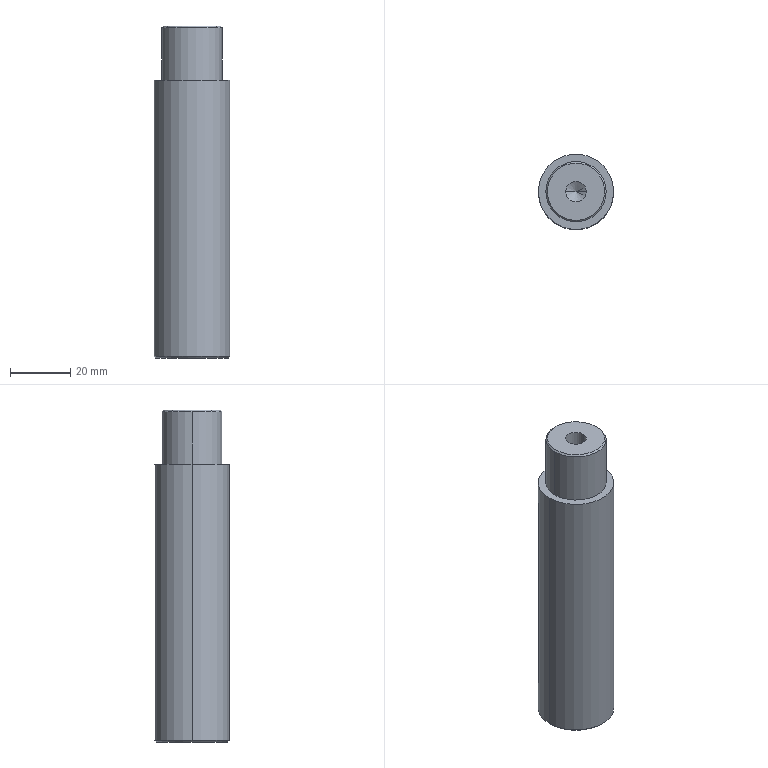Part | STEP file | 11-FG-Z00411 | 1 solid | 19 faces | box 25 x 25 x 110 mm | volume 49310 mm3 | cone 8 | cylinder 8 | plane 3 | commonest cylinder face diameters 6.8 x4 20 x2 25 x2
STEP:
#1=CARTESIAN_POINT('',(-12.,0.,0.));
#2=VERTEX_POINT('',#1);
#3=CARTESIAN_POINT('',(12.,0.,0.));
#4=VERTEX_POINT('',#3);
#5=CARTESIAN_POINT('',(0.,0.,0.));
#6=DIRECTION('',(0.,0.,-1.));
#7=DIRECTION('',(1.,0.,0.));
#8=AXIS2_PLACEMENT_3D('',#5,#6,#7);
#9=CIRCLE('',#8,12.);
#10=EDGE_CURVE('',#2,#4,#9,.T.);
#11=ORIENTED_EDGE('',*,*,#10,.F.);
#12=CARTESIAN_POINT('',(-12.5,0.,0.5));
#13=VERTEX_POINT('',#12);
#14=CARTESIAN_POINT('',(-12.5,0.,0.5));
#15=DIRECTION('',(-0.7071,0.,0.7071));
#16=VECTOR('',#15,1000.);
#17=LINE('',#14,#16);
#18=EDGE_CURVE('',#2,#13,#17,.T.);
#19=ORIENTED_EDGE('',*,*,#18,.T.);
#20=CARTESIAN_POINT('',(12.5,0.,0.5));
#21=VERTEX_POINT('',#20);
#22=CARTESIAN_POINT('',(0.,0.,0.5));
#23=DIRECTION('',(0.,0.,1.));
#24=DIRECTION('',(1.,0.,0.));
#25=AXIS2_PLACEMENT_3D('',#22,#23,#24);
#26=CIRCLE('',#25,12.5);
#27=EDGE_CURVE('',#21,#13,#26,.T.);
#28=ORIENTED_EDGE('',*,*,#27,.F.);
#29=CARTESIAN_POINT('',(12.5,0.,0.5));
#30=DIRECTION('',(0.7071,0.,0.7071));
#31=VECTOR('',#30,1000.);
#32=LINE('',#29,#31);
#33=EDGE_CURVE('',#4,#21,#32,.T.);
#34=ORIENTED_EDGE('',*,*,#33,.F.);
#35=EDGE_LOOP('',(#11,#19,#28,#34));
#36=FACE_OUTER_BOUND('',#35,.T.);
#37=CARTESIAN_POINT('',(0.,0.,0.5));
#38=DIRECTION('',(0.,0.,1.));
#39=DIRECTION('',(1.,0.,0.));
#40=AXIS2_PLACEMENT_3D('',#37,#38,#39);
#41=CONICAL_SURFACE('',#40,12.5,0.7854);
#42=ADVANCED_FACE('',(#36),#41,.T.);
#43=CARTESIAN_POINT('',(9.5,0.,110.));
#44=VERTEX_POINT('',#43);
#45=CARTESIAN_POINT('',(-9.5,0.,110.));
#46=VERTEX_POINT('',#45);
#47=CARTESIAN_POINT('',(0.,0.,110.));
#48=DIRECTION('',(0.,0.,1.));
#49=DIRECTION('',(1.,0.,0.));
#50=AXIS2_PLACEMENT_3D('',#47,#48,#49);
#51=CIRCLE('',#50,9.5);
#52=EDGE_CURVE('',#44,#46,#51,.T.);
#53=ORIENTED_EDGE('',*,*,#52,.F.);
#54=CARTESIAN_POINT('',(10.,0.,109.5));
#55=VERTEX_POINT('',#54);
#56=CARTESIAN_POINT('',(9.5,0.,110.));
#57=DIRECTION('',(0.7071,0.,-0.7071));
#58=VECTOR('',#57,1000.);
#59=LINE('',#56,#58);
#60=EDGE_CURVE('',#44,#55,#59,.T.);
#61=ORIENTED_EDGE('',*,*,#60,.T.);
#62=CARTESIAN_POINT('',(-10.,0.,109.5));
#63=VERTEX_POINT('',#62);
#64=CARTESIAN_POINT('',(0.,0.,109.5));
#65=DIRECTION('',(0.,0.,-1.));
#66=DIRECTION('',(1.,0.,0.));
#67=AXIS2_PLACEMENT_3D('',#64,#65,#66);
#68=CIRCLE('',#67,10.);
#69=EDGE_CURVE('',#63,#55,#68,.T.);
#70=ORIENTED_EDGE('',*,*,#69,.F.);
#71=CARTESIAN_POINT('',(-9.5,0.,110.));
#72=DIRECTION('',(-0.7071,0.,-0.7071));
#73=VECTOR('',#72,1000.);
#74=LINE('',#71,#73);
#75=EDGE_CURVE('',#46,#63,#74,.T.);
#76=ORIENTED_EDGE('',*,*,#75,.F.);
#77=EDGE_LOOP('',(#53,#61,#70,#76));
#78=FACE_OUTER_BOUND('',#77,.T.);
#79=CARTESIAN_POINT('',(0.,0.,110.));
#80=DIRECTION('',(0.,0.,-1.));
#81=DIRECTION('',(-1.,0.,0.));
#82=AXIS2_PLACEMENT_3D('',#79,#80,#81);
#83=CONICAL_SURFACE('',#82,9.5,0.7854);
#84=ADVANCED_FACE('',(#78),#83,.T.);
#85=CARTESIAN_POINT('',(-3.4,0.,90.2));
#86=VERTEX_POINT('',#85);
#87=CARTESIAN_POINT('',(3.4,0.,90.2));
#88=VERTEX_POINT('',#87);
#89=CARTESIAN_POINT('',(0.,0.,90.2));
#90=DIRECTION('',(0.,0.,1.));
#91=DIRECTION('',(1.,0.,0.));
#92=AXIS2_PLACEMENT_3D('',#89,#90,#91);
#93=CIRCLE('',#92,3.4);
#94=EDGE_CURVE('',#86,#88,#93,.T.);
#95=ORIENTED_EDGE('',*,*,#94,.F.);
#96=CARTESIAN_POINT('',(-3.4,0.,110.));
#97=VERTEX_POINT('',#96);
#98=CARTESIAN_POINT('',(-3.4,0.,110.));
#99=DIRECTION('',(0.,0.,1.));
#100=VECTOR('',#99,1000.);
#101=LINE('',#98,#100);
#102=EDGE_CURVE('',#86,#97,#101,.T.);
#103=ORIENTED_EDGE('',*,*,#102,.T.);
#104=CARTESIAN_POINT('',(3.4,0.,110.));
#105=VERTEX_POINT('',#104);
#106=CARTESIAN_POINT('',(0.,0.,110.));
#107=DIRECTION('',(0.,0.,1.));
#108=DIRECTION('',(1.,0.,0.));
#109=AXIS2_PLACEMENT_3D('',#106,#107,#108);
#110=CIRCLE('',#109,3.4);
#111=EDGE_CURVE('',#97,#105,#110,.T.);
#112=ORIENTED_EDGE('',*,*,#111,.T.);
#113=CARTESIAN_POINT('',(3.4,0.,110.));
#114=DIRECTION('',(0.,0.,1.));
#115=VECTOR('',#114,1000.);
#116=LINE('',#113,#115);
#117=EDGE_CURVE('',#88,#105,#116,.T.);
#118=ORIENTED_EDGE('',*,*,#117,.F.);
#119=EDGE_LOOP('',(#95,#103,#112,#118));
#120=FACE_OUTER_BOUND('',#119,.T.);
#121=CARTESIAN_POINT('',(0.,0.,110.));
#122=DIRECTION('',(0.,0.,1.));
#123=DIRECTION('',(1.,0.,0.));
#124=AXIS2_PLACEMENT_3D('',#121,#122,#123);
#125=CYLINDRICAL_SURFACE('',#124,3.4);
#126=ADVANCED_FACE('',(#120),#125,.F.);
#127=CARTESIAN_POINT('',(0.,0.,88.157));
#128=VERTEX_POINT('',#127);
#129=CARTESIAN_POINT('',(3.4,0.,90.2));
#130=DIRECTION('',(0.8572,0.,0.515));
#131=VECTOR('',#130,1000.);
#132=LINE('',#129,#131);
#133=EDGE_CURVE('',#128,#88,#132,.T.);
#134=ORIENTED_EDGE('',*,*,#133,.F.);
#135=CARTESIAN_POINT('',(-3.4,0.,90.2));
#136=DIRECTION('',(-0.8572,0.,0.515));
#137=VECTOR('',#136,1000.);
#138=LINE('',#135,#137);
#139=EDGE_CURVE('',#128,#86,#138,.T.);
#140=ORIENTED_EDGE('',*,*,#139,.T.);
#141=ORIENTED_EDGE('',*,*,#94,.T.);
#142=EDGE_LOOP('',(#134,#140,#141));
#143=FACE_OUTER_BOUND('',#142,.T.);
#144=CARTESIAN_POINT('',(0.,0.,90.2));
#145=DIRECTION('',(0.,0.,1.));
#146=DIRECTION('',(1.,0.,0.));
#147=AXIS2_PLACEMENT_3D('',#144,#145,#146);
#148=CONICAL_SURFACE('',#147,3.4,1.03);
#149=ADVANCED_FACE('',(#143),#148,.F.);
#150=CARTESIAN_POINT('',(10.,0.,92.));
#151=VERTEX_POINT('',#150);
#152=CARTESIAN_POINT('',(-10.,0.,92.));
#153=VERTEX_POINT('',#152);
#154=CARTESIAN_POINT('',(0.,0.,92.));
#155=DIRECTION('',(0.,0.,1.));
#156=DIRECTION('',(1.,0.,0.));
#157=AXIS2_PLACEMENT_3D('',#154,#155,#156);
#158=CIRCLE('',#157,10.);
#159=EDGE_CURVE('',#151,#153,#158,.T.);
#160=ORIENTED_EDGE('',*,*,#159,.T.);
#161=CARTESIAN_POINT('',(-10.,0.,92.));
#162=DIRECTION('',(0.,0.,1.));
#163=VECTOR('',#162,1000.);
#164=LINE('',#161,#163);
#165=EDGE_CURVE('',#153,#63,#164,.T.);
#166=ORIENTED_EDGE('',*,*,#165,.T.);
#167=ORIENTED_EDGE('',*,*,#69,.T.);
#168=CARTESIAN_POINT('',(10.,0.,92.));
#169=DIRECTION('',(0.,0.,1.));
#170=VECTOR('',#169,1000.);
#171=LINE('',#168,#170);
#172=EDGE_CURVE('',#151,#55,#171,.T.);
#173=ORIENTED_EDGE('',*,*,#172,.F.);
#174=EDGE_LOOP('',(#160,#166,#167,#173));
#175=FACE_OUTER_BOUND('',#174,.T.);
#176=CARTESIAN_POINT('',(0.,0.,92.));
#177=DIRECTION('',(0.,0.,1.));
#178=DIRECTION('',(1.,0.,0.));
#179=AXIS2_PLACEMENT_3D('',#176,#177,#178);
#180=CYLINDRICAL_SURFACE('',#179,10.);
#181=ADVANCED_FACE('',(#175),#180,.T.);
#182=CARTESIAN_POINT('',(3.4,0.,19.8));
#183=VERTEX_POINT('',#182);
#184=CARTESIAN_POINT('',(-3.4,0.,19.8));
#185=VERTEX_POINT('',#184);
#186=CARTESIAN_POINT('',(0.,0.,19.8));
#187=DIRECTION('',(0.,0.,-1.));
#188=DIRECTION('',(-1.,0.,0.));
#189=AXIS2_PLACEMENT_3D('',#186,#187,#188);
#190=CIRCLE('',#189,3.4);
#191=EDGE_CURVE('',#183,#185,#190,.T.);
#192=ORIENTED_EDGE('',*,*,#191,.F.);
#193=CARTESIAN_POINT('',(3.4,0.,0.));
#194=VERTEX_POINT('',#193);
#195=CARTESIAN_POINT('',(3.4,0.,0.));
#196=DIRECTION('',(0.,0.,-1.));
#197=VECTOR('',#196,1000.);
#198=LINE('',#195,#197);
#199=EDGE_CURVE('',#183,#194,#198,.T.);
#200=ORIENTED_EDGE('',*,*,#199,.T.);
#201=CARTESIAN_POINT('',(-3.4,0.,0.));
#202=VERTEX_POINT('',#201);
#203=CARTESIAN_POINT('',(0.,0.,0.));
#204=DIRECTION('',(0.,0.,-1.));
#205=DIRECTION('',(-1.,0.,0.));
#206=AXIS2_PLACEMENT_3D('',#203,#204,#205);
#207=CIRCLE('',#206,3.4);
#208=EDGE_CURVE('',#194,#202,#207,.T.);
#209=ORIENTED_EDGE('',*,*,#208,.T.);
#210=CARTESIAN_POINT('',(-3.4,0.,0.));
#211=DIRECTION('',(0.,0.,-1.));
#212=VECTOR('',#211,1000.);
#213=LINE('',#210,#212);
#214=EDGE_CURVE('',#185,#202,#213,.T.);
#215=ORIENTED_EDGE('',*,*,#214,.F.);
#216=EDGE_LOOP('',(#192,#200,#209,#215));
#217=FACE_OUTER_BOUND('',#216,.T.);
#218=CARTESIAN_POINT('',(0.,0.,0.));
#219=DIRECTION('',(0.,0.,-1.));
#220=DIRECTION('',(-1.,0.,0.));
#221=AXIS2_PLACEMENT_3D('',#218,#219,#220);
#222=CYLINDRICAL_SURFACE('',#221,3.4);
#223=ADVANCED_FACE('',(#217),#222,.F.);
#224=CARTESIAN_POINT('',(0.,0.,21.843));
#225=VERTEX_POINT('',#224);
#226=CARTESIAN_POINT('',(-3.4,0.,19.8));
#227=DIRECTION('',(-0.8572,0.,-0.515));
#228=VECTOR('',#227,1000.);
#229=LINE('',#226,#228);
#230=EDGE_CURVE('',#225,#185,#229,.T.);
#231=ORIENTED_EDGE('',*,*,#230,.F.);
#232=CARTESIAN_POINT('',(3.4,0.,19.8));
#233=DIRECTION('',(0.8572,0.,-0.515));
#234=VECTOR('',#233,1000.);
#235=LINE('',#232,#234);
#236=EDGE_CURVE('',#225,#183,#235,.T.);
#237=ORIENTED_EDGE('',*,*,#236,.T.);
#238=ORIENTED_EDGE('',*,*,#191,.T.);
#239=EDGE_LOOP('',(#231,#237,#238));
#240=FACE_OUTER_BOUND('',#239,.T.);
#241=CARTESIAN_POINT('',(0.,0.,19.8));
#242=DIRECTION('',(0.,0.,-1.));
#243=DIRECTION('',(-1.,0.,0.));
#244=AXIS2_PLACEMENT_3D('',#241,#242,#243);
#245=CONICAL_SURFACE('',#244,3.4,1.03);
#246=ADVANCED_FACE('',(#240),#245,.F.);
#247=CARTESIAN_POINT('',(12.5,0.,92.));
#248=VERTEX_POINT('',#247);
#249=CARTESIAN_POINT('',(-12.5,0.,92.));
#250=VERTEX_POINT('',#249);
#251=CARTESIAN_POINT('',(0.,0.,92.));
#252=DIRECTION('',(0.,0.,1.));
#253=DIRECTION('',(1.,0.,0.));
#254=AXIS2_PLACEMENT_3D('',#251,#252,#253);
#255=CIRCLE('',#254,12.5);
#256=EDGE_CURVE('',#248,#250,#255,.T.);
#257=ORIENTED_EDGE('',*,*,#256,.F.);
#258=CARTESIAN_POINT('',(12.5,0.,110.));
#259=DIRECTION('',(0.,0.,-1.));
#260=VECTOR('',#259,1000.);
#261=LINE('',#258,#260);
#262=EDGE_CURVE('',#248,#21,#261,.T.);
#263=ORIENTED_EDGE('',*,*,#262,.T.);
#264=ORIENTED_EDGE('',*,*,#27,.T.);
#265=CARTESIAN_POINT('',(-12.5,0.,110.));
#266=DIRECTION('',(0.,0.,-1.));
#267=VECTOR('',#266,1000.);
#268=LINE('',#265,#267);
#269=EDGE_CURVE('',#250,#13,#268,.T.);
#270=ORIENTED_EDGE('',*,*,#269,.F.);
#271=EDGE_LOOP('',(#257,#263,#264,#270));
#272=FACE_OUTER_BOUND('',#271,.T.);
#273=CARTESIAN_POINT('',(0.,0.,110.));
#274=DIRECTION('',(0.,0.,-1.));
#275=DIRECTION('',(-1.,0.,0.));
#276=AXIS2_PLACEMENT_3D('',#273,#274,#275);
#277=CYLINDRICAL_SURFACE('',#276,12.5);
#278=ADVANCED_FACE('',(#272),#277,.T.);
#279=ORIENTED_EDGE('',*,*,#262,.F.);
#280=CARTESIAN_POINT('',(0.,0.,92.));
#281=DIRECTION('',(0.,0.,1.));
#282=DIRECTION('',(1.,0.,0.));
#283=AXIS2_PLACEMENT_3D('',#280,#281,#282);
#284=CIRCLE('',#283,12.5);
#285=EDGE_CURVE('',#250,#248,#284,.T.);
#286=ORIENTED_EDGE('',*,*,#285,.F.);
#287=ORIENTED_EDGE('',*,*,#269,.T.);
#288=CARTESIAN_POINT('',(0.,0.,0.5));
#289=DIRECTION('',(0.,0.,1.));
#290=DIRECTION('',(1.,0.,0.));
#291=AXIS2_PLACEMENT_3D('',#288,#289,#290);
#292=CIRCLE('',#291,12.5);
#293=EDGE_CURVE('',#13,#21,#292,.T.);
#294=ORIENTED_EDGE('',*,*,#293,.T.);
#295=EDGE_LOOP('',(#279,#286,#287,#294));
#296=FACE_OUTER_BOUND('',#295,.T.);
#297=CARTESIAN_POINT('',(0.,0.,110.));
#298=DIRECTION('',(0.,0.,-1.));
#299=DIRECTION('',(-1.,0.,0.));
#300=AXIS2_PLACEMENT_3D('',#297,#298,#299);
#301=CYLINDRICAL_SURFACE('',#300,12.5);
#302=ADVANCED_FACE('',(#296),#301,.T.);
#303=CARTESIAN_POINT('',(0.,0.,0.));
#304=DIRECTION('',(0.,0.,-1.));
#305=DIRECTION('',(1.,0.,0.));
#306=AXIS2_PLACEMENT_3D('',#303,#304,#305);
#307=CIRCLE('',#306,12.);
#308=EDGE_CURVE('',#4,#2,#307,.T.);
#309=ORIENTED_EDGE('',*,*,#308,.T.);
#310=ORIENTED_EDGE('',*,*,#10,.T.);
#311=EDGE_LOOP('',(#309,#310));
#312=FACE_OUTER_BOUND('',#311,.T.);
#313=CARTESIAN_POINT('',(0.,0.,0.));
#314=DIRECTION('',(0.,0.,-1.));
#315=DIRECTION('',(-1.,0.,0.));
#316=AXIS2_PLACEMENT_3D('',#313,#314,#315);
#317=CIRCLE('',#316,3.4);
#318=EDGE_CURVE('',#202,#194,#317,.T.);
#319=ORIENTED_EDGE('',*,*,#318,.F.);
#320=ORIENTED_EDGE('',*,*,#208,.F.);
#321=EDGE_LOOP('',(#319,#320));
#322=FACE_BOUND('',#321,.T.);
#323=CARTESIAN_POINT('',(0.,0.,0.));
#324=DIRECTION('',(0.,0.,1.));
#325=DIRECTION('',(1.,0.,0.));
#326=AXIS2_PLACEMENT_3D('',#323,#324,#325);
#327=PLANE('',#326);
#328=ADVANCED_FACE('',(#312,#322),#327,.F.);
#329=ORIENTED_EDGE('',*,*,#236,.F.);
#330=ORIENTED_EDGE('',*,*,#230,.T.);
#331=CARTESIAN_POINT('',(0.,0.,19.8));
#332=DIRECTION('',(0.,0.,-1.));
#333=DIRECTION('',(-1.,0.,0.));
#334=AXIS2_PLACEMENT_3D('',#331,#332,#333);
#335=CIRCLE('',#334,3.4);
#336=EDGE_CURVE('',#185,#183,#335,.T.);
#337=ORIENTED_EDGE('',*,*,#336,.T.);
#338=EDGE_LOOP('',(#329,#330,#337));
#339=FACE_OUTER_BOUND('',#338,.T.);
#340=CARTESIAN_POINT('',(0.,0.,19.8));
#341=DIRECTION('',(0.,0.,-1.));
#342=DIRECTION('',(-1.,0.,0.));
#343=AXIS2_PLACEMENT_3D('',#340,#341,#342);
#344=CONICAL_SURFACE('',#343,3.4,1.03);
#345=ADVANCED_FACE('',(#339),#344,.F.);
#346=ORIENTED_EDGE('',*,*,#199,.F.);
#347=ORIENTED_EDGE('',*,*,#336,.F.);
#348=ORIENTED_EDGE('',*,*,#214,.T.);
#349=ORIENTED_EDGE('',*,*,#318,.T.);
#350=EDGE_LOOP('',(#346,#347,#348,#349));
#351=FACE_OUTER_BOUND('',#350,.T.);
#352=CARTESIAN_POINT('',(0.,0.,0.));
#353=DIRECTION('',(0.,0.,-1.));
#354=DIRECTION('',(-1.,0.,0.));
#355=AXIS2_PLACEMENT_3D('',#352,#353,#354);
#356=CYLINDRICAL_SURFACE('',#355,3.4);
#357=ADVANCED_FACE('',(#351),#356,.F.);
#358=ORIENTED_EDGE('',*,*,#159,.F.);
#359=CARTESIAN_POINT('',(0.,0.,92.));
#360=DIRECTION('',(0.,0.,1.));
#361=DIRECTION('',(1.,0.,0.));
#362=AXIS2_PLACEMENT_3D('',#359,#360,#361);
#363=CIRCLE('',#362,10.);
#364=EDGE_CURVE('',#153,#151,#363,.T.);
#365=ORIENTED_EDGE('',*,*,#364,.F.);
#366=EDGE_LOOP('',(#358,#365));
#367=FACE_BOUND('',#366,.T.);
#368=ORIENTED_EDGE('',*,*,#285,.T.);
#369=ORIENTED_EDGE('',*,*,#256,.T.);
#370=EDGE_LOOP('',(#368,#369));
#371=FACE_OUTER_BOUND('',#370,.T.);
#372=CARTESIAN_POINT('',(0.,0.,92.));
#373=DIRECTION('',(0.,0.,1.));
#374=DIRECTION('',(1.,0.,0.));
#375=AXIS2_PLACEMENT_3D('',#372,#373,#374);
#376=PLANE('',#375);
#377=ADVANCED_FACE('',(#367,#371),#376,.T.);
#378=ORIENTED_EDGE('',*,*,#165,.F.);
#379=ORIENTED_EDGE('',*,*,#364,.T.);
#380=ORIENTED_EDGE('',*,*,#172,.T.);
#381=CARTESIAN_POINT('',(0.,0.,109.5));
#382=DIRECTION('',(0.,0.,-1.));
#383=DIRECTION('',(1.,0.,0.));
#384=AXIS2_PLACEMENT_3D('',#381,#382,#383);
#385=CIRCLE('',#384,10.);
#386=EDGE_CURVE('',#55,#63,#385,.T.);
#387=ORIENTED_EDGE('',*,*,#386,.T.);
#388=EDGE_LOOP('',(#378,#379,#380,#387));
#389=FACE_OUTER_BOUND('',#388,.T.);
#390=CARTESIAN_POINT('',(0.,0.,92.));
#391=DIRECTION('',(0.,0.,1.));
#392=DIRECTION('',(1.,0.,0.));
#393=AXIS2_PLACEMENT_3D('',#390,#391,#392);
#394=CYLINDRICAL_SURFACE('',#393,10.);
#395=ADVANCED_FACE('',(#389),#394,.T.);
#396=ORIENTED_EDGE('',*,*,#139,.F.);
#397=ORIENTED_EDGE('',*,*,#133,.T.);
#398=CARTESIAN_POINT('',(0.,0.,90.2));
#399=DIRECTION('',(0.,0.,1.));
#400=DIRECTION('',(1.,0.,0.));
#401=AXIS2_PLACEMENT_3D('',#398,#399,#400);
#402=CIRCLE('',#401,3.4);
#403=EDGE_CURVE('',#88,#86,#402,.T.);
#404=ORIENTED_EDGE('',*,*,#403,.T.);
#405=EDGE_LOOP('',(#396,#397,#404));
#406=FACE_OUTER_BOUND('',#405,.T.);
#407=CARTESIAN_POINT('',(0.,0.,90.2));
#408=DIRECTION('',(0.,0.,1.));
#409=DIRECTION('',(1.,0.,0.));
#410=AXIS2_PLACEMENT_3D('',#407,#408,#409);
#411=CONICAL_SURFACE('',#410,3.4,1.03);
#412=ADVANCED_FACE('',(#406),#411,.F.);
#413=ORIENTED_EDGE('',*,*,#102,.F.);
#414=ORIENTED_EDGE('',*,*,#403,.F.);
#415=ORIENTED_EDGE('',*,*,#117,.T.);
#416=CARTESIAN_POINT('',(0.,0.,110.));
#417=DIRECTION('',(0.,0.,1.));
#418=DIRECTION('',(1.,0.,0.));
#419=AXIS2_PLACEMENT_3D('',#416,#417,#418);
#420=CIRCLE('',#419,3.4);
#421=EDGE_CURVE('',#105,#97,#420,.T.);
#422=ORIENTED_EDGE('',*,*,#421,.T.);
#423=EDGE_LOOP('',(#413,#414,#415,#422));
#424=FACE_OUTER_BOUND('',#423,.T.);
#425=CARTESIAN_POINT('',(0.,0.,110.));
#426=DIRECTION('',(0.,0.,1.));
#427=DIRECTION('',(1.,0.,0.));
#428=AXIS2_PLACEMENT_3D('',#425,#426,#427);
#429=CYLINDRICAL_SURFACE('',#428,3.4);
#430=ADVANCED_FACE('',(#424),#429,.F.);
#431=CARTESIAN_POINT('',(0.,0.,110.));
#432=DIRECTION('',(0.,0.,1.));
#433=DIRECTION('',(1.,0.,0.));
#434=AXIS2_PLACEMENT_3D('',#431,#432,#433);
#435=CIRCLE('',#434,9.5);
#436=EDGE_CURVE('',#46,#44,#435,.T.);
#437=ORIENTED_EDGE('',*,*,#436,.T.);
#438=ORIENTED_EDGE('',*,*,#52,.T.);
#439=EDGE_LOOP('',(#437,#438));
#440=FACE_OUTER_BOUND('',#439,.T.);
#441=ORIENTED_EDGE('',*,*,#421,.F.);
#442=ORIENTED_EDGE('',*,*,#111,.F.);
#443=EDGE_LOOP('',(#441,#442));
#444=FACE_BOUND('',#443,.T.);
#445=CARTESIAN_POINT('',(0.,0.,110.));
#446=DIRECTION('',(0.,0.,1.));
#447=DIRECTION('',(1.,0.,0.));
#448=AXIS2_PLACEMENT_3D('',#445,#446,#447);
#449=PLANE('',#448);
#450=ADVANCED_FACE('',(#440,#444),#449,.T.);
#451=ORIENTED_EDGE('',*,*,#60,.F.);
#452=ORIENTED_EDGE('',*,*,#436,.F.);
#453=ORIENTED_EDGE('',*,*,#75,.T.);
#454=ORIENTED_EDGE('',*,*,#386,.F.);
#455=EDGE_LOOP('',(#451,#452,#453,#454));
#456=FACE_OUTER_BOUND('',#455,.T.);
#457=CARTESIAN_POINT('',(0.,0.,110.));
#458=DIRECTION('',(0.,0.,-1.));
#459=DIRECTION('',(-1.,0.,0.));
#460=AXIS2_PLACEMENT_3D('',#457,#458,#459);
#461=CONICAL_SURFACE('',#460,9.5,0.7854);
#462=ADVANCED_FACE('',(#456),#461,.T.);
#463=ORIENTED_EDGE('',*,*,#18,.F.);
#464=ORIENTED_EDGE('',*,*,#308,.F.);
#465=ORIENTED_EDGE('',*,*,#33,.T.);
#466=ORIENTED_EDGE('',*,*,#293,.F.);
#467=EDGE_LOOP('',(#463,#464,#465,#466));
#468=FACE_OUTER_BOUND('',#467,.T.);
#469=CARTESIAN_POINT('',(0.,0.,0.5));
#470=DIRECTION('',(0.,0.,1.));
#471=DIRECTION('',(1.,0.,0.));
#472=AXIS2_PLACEMENT_3D('',#469,#470,#471);
#473=CONICAL_SURFACE('',#472,12.5,0.7854);
#474=ADVANCED_FACE('',(#468),#473,.T.);
#475=CLOSED_SHELL('',(#42,#84,#126,#149,#181,#223,#246,#278,#302,#328,#345,#357,#377,#395,#412,#430,#450,#462,#474));
#476=MANIFOLD_SOLID_BREP('',#475);
#477=CARTESIAN_POINT('',(0.,0.,0.));
#478=DIRECTION('',(0.,0.,1.));
#479=DIRECTION('',(1.,0.,0.));
#480=AXIS2_PLACEMENT_3D('',#477,#478,#479);
#481=(LENGTH_UNIT()NAMED_UNIT(*)SI_UNIT(.MILLI.,.METRE.));
#482=UNCERTAINTY_MEASURE_WITH_UNIT(LENGTH_MEASURE(0.00001),#481,'','');
#483=(NAMED_UNIT(*)PLANE_ANGLE_UNIT()SI_UNIT($,.RADIAN.));
#484=(NAMED_UNIT(*)SI_UNIT($,.STERADIAN.)SOLID_ANGLE_UNIT());
#485=(GEOMETRIC_REPRESENTATION_CONTEXT(3)GLOBAL_UNCERTAINTY_ASSIGNED_CONTEXT((#482))GLOBAL_UNIT_ASSIGNED_CONTEXT((#481,#483,#484))REPRESENTATION_CONTEXT('',''));
#486=ADVANCED_BREP_SHAPE_REPRESENTATION('',(#476,#480),#485);